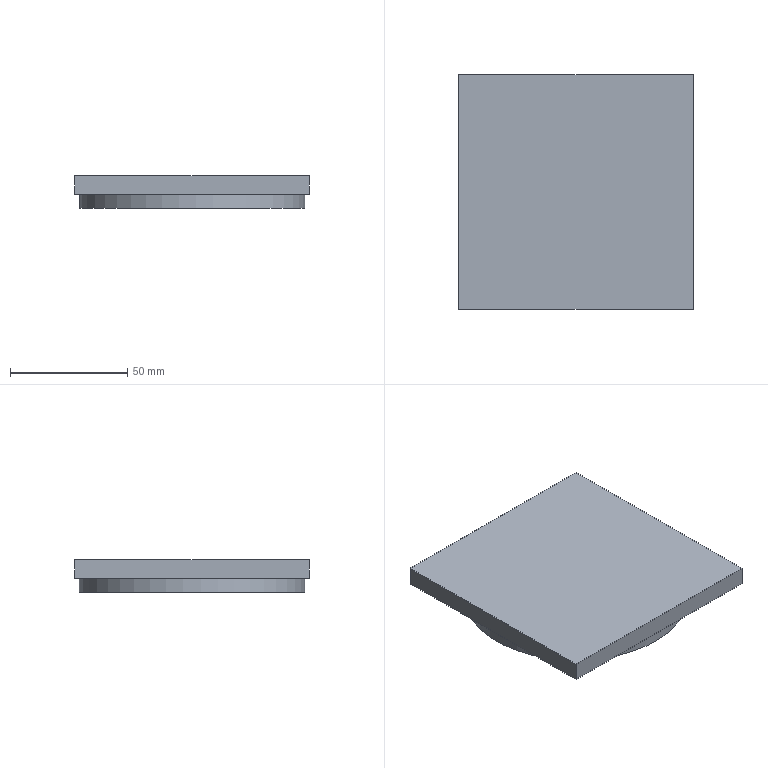NC program | NX | posted with a generic post | part box 100 x 100 x 14 mm
Whole program:
N10 G17 G21 G94 G90
(ADAPTIVE_MILLING_2 , TOOL : D-12)
N12 T02 M6
N14 G54
N16 G17 G0 G90 X-3.154 Y4.386 S4500 M3
N18 G43 Z10.1 H2
N20 Z3.
N22 G94 G3 X-3.154 Y4.386 Z2.408 I3.153 J-4.384 F2000.
N24 X-3.154 Y4.386 Z1.816 I3.153 J-4.384
N26 X-3.154 Y4.386 Z1.223 I3.153 J-4.384
N28 X-3.154 Y4.386 Z0.631 I3.153 J-4.384
N30 X-3.154 Y4.386 Z0.039 I3.153 J-4.384
N32 X-3.154 Y4.386 Z-0.553 I3.153 J-4.384
N34 X-3.154 Y4.386 Z-1.146 I3.153 J-4.384
N36 X-3.154 Y4.386 Z-1.738 I3.153 J-4.384
N38 X-3.154 Y4.386 Z-2.33 I3.153 J-4.384
N40 X-3.154 Y4.386 Z-2.922 I3.153 J-4.384
N42 X-3.154 Y4.386 Z-3.515 I3.153 J-4.384
N44 X5.399 Y0.003 Z-3.9 R-5.4
N46 X-1.557 Y-5.214 R-5.422
N48 X4.806 Y-2.622 R5.524
N50 X0.599 Y5.862 R5.572
N52 X3.914 Y-4.46 R-5.914
N54 X3.84 Y5.052 R6.148
N56 X-6.148 Y-1.842 R6.369
N58 X4.805 Y-4.324 R6.465
N60 X-1.857 Y6.664 R6.659
N62 X3.83 Y-5.821 R-6.942
N64 X-2.133 Y7.148 R7.204
N66 X3.422 Y-6.682 R-7.483
N68 X-2.192 Y7.708 R7.755
N70 X3.004 Y-7.488 R-8.041
N72 X-2.328 Y8.263 R8.325
N74 X2.608 Y-8.242 R-8.615
N76 X-1.916 Y8.963 R8.904
N78 X1.279 Y-9.143 R9.199
N80 X-1.232 Y9.692 R9.501
N82 X0.279 Y-9.83 R9.801
N84 X0.09 Y10.38 R10.107
N86 X-0.3 Y-10.454 R10.419
N88 X2.062 Y10.798 R10.728
N90 X-8.38 Y-7.238 R11.022
N92 X10.545 Y-3.97 R11.233
N94 X-5.824 Y10.126 R11.433
N96 X0.432 Y-11.743 R11.716
N98 X2.752 Y11.976 R12.024
N100 X-9.497 Y-7.947 R12.323
N102 X11.764 Y-4.48 R12.551
N104 X-5.301 Y11.881 R12.759
N106 X-0.296 Y-13.081 R13.048
N108 X6.412 Y11.99 R13.354
N110 X-13.728 Y-0.149 R13.626
N112 X8.106 Y-11.22 R13.819
N114 X-0.309 Y14.351 R14.088
N116 X-6.106 Y-13.092 R14.395
N118 X14.563 Y2.568 R14.679
N120 X-10.027 Y11.288 R14.878
N122 X0.527 Y-15.17 R15.144
N124 X6.903 Y14.099 R15.452
N126 X-15.656 Y2.387 R15.723
N128 X7.333 Y-14.153 R15.911
N130 X3.483 Y16.083 R16.198
N132 X-15.995 Y-4.32 R16.482
N134 X12.489 Y-11.121 R16.687
N136 X2.015 Y17.079 R16.945
N138 X-14.965 Y-8.694 R17.233
N140 X16.444 Y-6.093 R17.478
N142 X-8.037 Y16.085 R17.72
N144 X-3.613 Y-17.706 R18.027
N146 X15.402 Y10.258 R18.322
N148 X-15.46 Y10.611 R18.562
N150 X-0.924 Y-18.808 R18.802
N152 X13.901 Y13.378 R19.087
N154 X-17.673 Y8.259 R19.332
N156 X0.474 Y-19.588 R19.571
N158 X12.623 Y15.608 R19.854
N160 X-17.823 Y9.643 R20.089
N162 X-0.493 Y-20.345 R20.328
N164 X15.558 Y13.8 R20.598
N166 X-16.806 Y12.636 R20.828
N168 X0.095 Y-21.118 R21.089
N170 X18.388 Y11.193 R21.358
N172 X-19.11 Y10.49 R21.602
N174 X1.325 Y-21.861 R21.873
N176 X19.105 Y11.502 R22.14
N178 X-19.843 Y10.765 R22.375
N180 X1.168 Y-22.652 R22.651
N182 X18.905 Y13.264 R22.925
N184 X-20.402 Y11.372 R23.157
N186 X0.635 Y-23.458 R23.439
N188 X20.591 Y12.053 R23.704
N190 X-21.553 Y10.879 R23.938
N192 X-0.268 Y-24.254 R24.231
N194 X23.762 Y6.301 R24.464
N196 X-20.649 Y13.973 R24.707
N198 X-2.624 Y-24.902 R25.014
N200 X25.289 Y-0.95 R25.215
N202 X-18.779 Y17.576 R25.473
N204 X-6.417 Y-25.012 R25.79
N206 X25.957 Y-2.636 R25.987
N208 X-19.48 Y18.005 R26.275
N210 X-7.266 Y-25.616 R26.6
N212 X26.875 Y-1.259 R26.79
N214 X-20.758 Y17.78 R27.083
N216 X-8.934 Y-25.935 R27.403
N218 X27.721 Y-0.102 R27.594
N220 X-21.869 Y17.714 R27.894
N222 X-8.116 Y-27.063 R28.223
N224 X28.437 Y2.598 R28.427
N226 X-24.837 Y14.895 R28.721
N228 X-6.903 Y-28.247 R29.051
N230 X29.183 Y3.371 R29.242
N232 X-25.679 Y15.086 R29.542
N234 X-7.005 Y-29.07 R29.878
N236 X29.661 Y5.746 R30.071
N238 X-26.428 Y15.437 R30.365
N240 X-9.619 Y-29.174 R30.706
N242 X30.414 Y6.192 R30.886
N244 X-27.094 Y15.937 R31.196
N246 X-17.248 Y-26.373 R31.512
N248 X31.79 Y-1.503 R31.675
N250 X-27.025 Y17.624 R32.024
N252 X-16.339 Y-27.923 R32.355
N254 X32.668 Y0.441 R32.517
N256 X-28.532 Y16.778 R32.864
N258 X-2.21 Y-33.181 R33.22
N260 X30.276 Y14.534 R33.433
N262 X-31.561 Y12.486 R33.719
N264 X23.01 Y-25.322 R34.096
N266 X20.816 Y27.545 R34.406
N268 X-32.795 Y11.582 R34.569
N270 X24.639 Y-24.947 R34.939
N272 X17.473 Y30.781 R35.262
N274 X-35.279 Y4.959 R35.429
N276 X29.907 Y-19.934 R35.799
N278 X16.176 Y32.439 R36.137
N280 X-36.447 Y-1.326 R36.286
N282 X30.969 Y-19.864 R36.647
N284 X16.619 Y33.159 R36.98
N286 X-37.303 Y-1.07 R37.129
N288 X31.298 Y-20.91 R37.495
N290 X17.662 Y33.569 R37.821
N292 X-38.136 Y-1.492 R37.972
N294 X30.405 Y-23.586 R38.339
N296 X18.094 Y34.301 R38.658
N298 X-38.735 Y-4.681 R38.83
N300 X30.258 Y-25.126 R39.187
N302 X18.487 Y35.057 R39.504
N304 X-39.614 Y-4.548 R39.685
N306 X31.879 Y-24.479 R40.047
N308 X18.202 Y36.17 R40.366
N310 X-40.399 Y-5.18 R40.543
N312 X31.37 Y-26.471 R40.901
N314 X17.814 Y37.319 R41.217
N316 X-41.413 Y-3.817 R41.398
N318 X23.892 Y-34.379 R41.74
N320 X32.41 Y-26.554 R41.359
N322 X37.613 Y-18.455 R43.987
N324 X31.003 Y28.184 R41.955
N326 X12.199 Y40.084 R42.277
N328 X7.559 Y41.212 R43.703
N330 G1 X4.503 Y41.656
N332 X1.443 Y41.873
N334 X-1.627 Y41.867
N336 X-4.686 Y41.635
N338 G3 X-10.57 Y40.544 R48.84
N340 X-40.065 Y12.261 R41.986
N342 X-41.444 Y6.153 R47.559
N344 X-41.883 Y-1.15 R45.993
N346 X-37.597 Y-18.495 R42.514
N348 X-8.498 Y-41.028 R42.018
N350 X3.138 Y-41.781 R43.295
N352 X9.035 Y-40.914 R48.757
N354 X24.141 Y-34.246 R41.956
N356 X27.81 Y-31.337 R53.813
N358 X27.717 Y-29.448 R1.212
N360 G1 X26.472 Y-28.546
N362 X26.351 Y-28.458 Z-3.896
N364 X26.229 Y-28.37 Z-3.885
N366 X26.108 Y-28.282 Z-3.866
N368 X25.986 Y-28.194 Z-3.839
N370 X25.865 Y-28.106 Z-3.805
N372 X25.743 Y-28.018 Z-3.762
N374 X25.622 Y-27.93 Z-3.71
N376 X25.5 Y-27.842 Z-3.65
N378 X25.379 Y-27.754 Z-3.579
N380 X25.257 Y-27.666 Z-3.498
N382 X25.136 Y-27.578 Z-3.405
N384 X25.014 Y-27.49 Z-3.3
N386 X24.893 Y-27.402 Z-3.18
N388 X24.771 Y-27.314 Z-3.042
N390 X24.65 Y-27.226 Z-2.884
N392 X24.529 Y-27.138 Z-2.7
N394 X24.407 Y-27.05 Z-2.48
N396 X24.286 Y-26.962 Z-2.208
N398 X24.164 Y-26.874 Z-1.837
N400 X24.043 Y-26.786 Z-0.9
N402 G0 Z10.1
(FLOOR_FACING_2 , TOOL : D-12)
N404 X0. Y-5.9
N406 Z-4.
N408 G3 X5.9 Y0. R5.9 F1000.
N410 X0. Y-5.9 R-5.9
N412 G1 Y-14.9
N414 G3 X14.9 Y0. R14.9
N416 X0. Y-14.9 R-14.9
N418 G1 Y-23.9
N420 G3 X23.9 Y0. R23.9
N422 X0. Y-23.9 R-23.9
N424 G1 Y-32.9
N426 G3 X32.9 Y0. R32.9
N428 X0. Y-32.9 R-32.9
N430 G1 Y-41.9
N432 G3 X41.9 Y0. R41.9
N434 X0. Y-41.9 R-41.9
N436 X1. Y-41.888 R41.9
N438 G1 Z-1.
N440 G0 Z10.1
(PLANAR_MILL_4 , TOOL : D-12)
N442 X38.995 Y-1.826
N444 Z10.02
N446 Z-1.
N448 G1 Z-4. F500.
N450 G41 X39.98 Y-2. D2
N452 G3 X41.98 Y0. R2.
N454 X0. Y41.98 R41.98
N456 X41.98 Y0. R-41.98
N458 X41.968 Y1. R41.98
N460 X39.921 Y2.952 R2.
N462 G40
N464 G1 X38.941 Y2.755
N466 Z2.
N468 G0 Z10.02
N470 M5
N472 M2